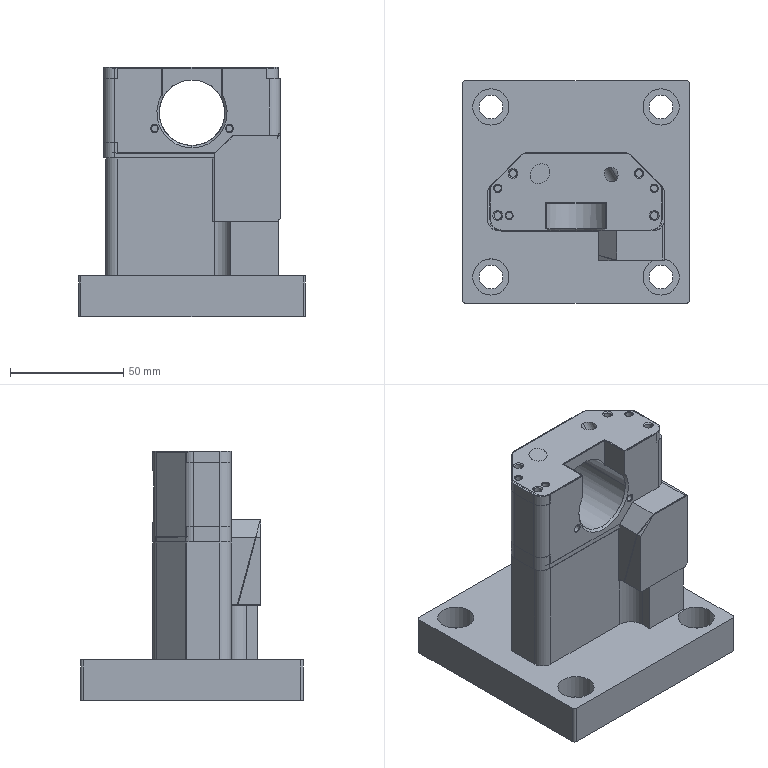NC program | NX | posted with a generic post | part box 100 x 98 x 110 mm
Whole program:
N10 G17 G21 G94 G90
(PLANAR_MILL , TOOL : D80面刀)
N12 T01 M6
N14 G53
N16 G17 G0 G90 X88. Y0. B0. C0. S3500 M3
N18 G43 Z30. H1
N20 Z2.05
N22 G94 G1 Z0.05 F800.
N24 X43.
N26 X-43.
N28 X-88.
N30 Z2.05
N32 G0 Z30.
N34 M5
(ADAPTIVE_MILLING , TOOL : D16-48-D16-100-3T-ROUGH)
N36 T02 M6
N38 G53
N40 G17 G0 G90 X-58.075 Y-25.19 B0. C0. S6500 M3
N42 G43 Z30. H2
N44 Z-24.9
N46 G94 G1 X-57.925 Y-25.183 Z-25.837 F2500.
N48 X-57.775 Y-25.177 Z-26.208
N50 X-57.625 Y-25.171 Z-26.48
N52 X-57.475 Y-25.164 Z-26.7
N54 X-57.325 Y-25.158 Z-26.884
N56 X-57.176 Y-25.152 Z-27.042
N58 X-57.026 Y-25.145 Z-27.18
N60 X-56.876 Y-25.139 Z-27.3
N62 X-56.726 Y-25.133 Z-27.405
N64 X-56.576 Y-25.126 Z-27.498
N66 X-56.426 Y-25.12 Z-27.579
N68 X-56.276 Y-25.114 Z-27.65
N70 X-56.127 Y-25.107 Z-27.71
N72 X-55.977 Y-25.101 Z-27.762
N74 X-55.827 Y-25.095 Z-27.805
N76 X-55.677 Y-25.088 Z-27.839
N78 X-55.527 Y-25.082 Z-27.866
N80 X-55.377 Y-25.075 Z-27.885
N82 X-55.227 Y-25.069 Z-27.896
N84 X-55.077 Y-25.063 Z-27.9
N86 X-52.483 Y-24.953
N88 G3 X-51.072 Y-23.99 R1.616
N90 X-50.404 Y-20.967 R10.918
N92 X-50.046 Y-12.897 R87.213
N94 X-50.001 Y0.166 R855.855
N96 G1 X-50. Y24.239
N98 G2 X-47.644 Y29.928 R8.523
N100 X-42.106 Y33.388 R13.172
N102 X-35.342 Y34.661 R28.151
N104 X-24.774 Y34.98 R145.286
N106 G1 X-12.324 Y34.999
N108 X39.312 Y34.998
N110 G2 X45.036 Y32.543 R8.577
N112 X48.435 Y26.964 R13.333
N114 X49.667 Y20.268 R28.64
N116 X49.98 Y9.775 R147.076
N118 G1 X49.999 Y-2.675
N120 Y-24.311
N122 G2 X47.693 Y-29.819 R8.552
N124 X42.228 Y-33.307 R13.103
N126 X35.398 Y-34.634 R27.707
N128 X24.906 Y-34.969 R139.792
N130 G1 X13.281 Y-34.991
N132 X-39.31 Y-34.998
N134 G2 X-45.115 Y-32.463 R8.58
N136 X-48.122 Y-27.095 R11.826
N138 X-48.966 Y-20.791 R27.513
N140 X-49.036 Y-15.842 R208.259
N142 G1 X-49.029 Y-1.961
N144 X-49.001 Y12.389
N146 G2 X-48.98 Y21.089 R508.483
N148 X-44.643 Y29.357 R11.495
N150 X-38.004 Y32.599 R17.441
N152 X-30.148 Y33.728 R40.171
N154 X-18.527 Y33.985 R219.275
N156 G1 X-8.627 Y33.998
N158 X35.561 Y33.997
N160 G2 X44.259 Y29.758 R11.447
N162 X47.559 Y23.15 R17.233
N164 X48.718 Y15.299 R39.324
N166 X48.986 Y3.079 R220.579
N168 G1 X48.998 Y-6.821
N170 X48.997 Y-20.486
N172 G2 X44.738 Y-29.238 R11.491
N174 X38.283 Y-32.496 R17.176
N176 X30.439 Y-33.693 R38.447
N178 X18.069 Y-33.977 R213.227
N180 G1 X8.169 Y-33.991
N182 X-35.56 Y-33.996
N184 G2 X-41.664 Y-31.998 R10.651
N186 G1 X-42.905 Y-31.48
N188 X-44.056 Y-30.775
N190 X-45.082 Y-29.898
N192 X-45.958 Y-28.872
N194 X-46.663 Y-27.721
N196 X-47.179 Y-26.475
N198 X-47.494 Y-25.162
N200 G2 X-48.002 Y-13.629 R123.608
N202 X-48.015 Y1.606 R886.218
N204 G1 X-48.003 Y10.291
N206 G2 X-47.968 Y18.213 R275.05
N208 X-42.166 Y28.601 R13.302
N210 X-35.036 Y31.664 R20.413
N212 X-26.49 Y32.748 R48.479
N214 X-13.293 Y32.989 R282.507
N216 G1 X-3.393 Y32.998
N218 X32.187 Y32.996
N220 G2 X39.553 Y31.028 R13.666
N222 X45.054 Y24.68 R14.976
N224 X47.217 Y17.129 R26.266
N226 X47.897 Y7.408 R80.681
N228 X47.998 Y-10.216 R882.689
N230 X47.973 Y-18.011 R320.297
N232 X42.252 Y-28.509 R13.323
N234 X35.139 Y-31.617 R20.267
N236 X26.898 Y-32.712 R46.807
N238 X13.252 Y-32.98 R265.456
N240 G1 X3.352 Y-32.991
N242 X-32.11 Y-32.995
N244 G2 X-36.486 Y-32.425 R18.992
N246 G1 X-39.001 Y-32.418
N248 X-40.346 Y-32.312
N250 X-41.728 Y-31.968
N252 X-40.346 Y-32.312
N254 X-39.001 Y-32.418
N256 X-9.236 Y-32.412
N258 X-0.282 Y-32.393
N260 X11.018 Y-32.384
N262 G3 X25.265 Y-32.164 R333.183
N264 X33.82 Y-31.154 R50.803
N266 X40.547 Y-28.463 R20.326
N268 X46.408 Y-20.132 R13.66
N270 X47.244 Y-13.748 R31.907
N272 X47.381 Y-0.7 R293.683
N274 X47.074 Y12.045 R211.801
N276 X45.853 Y20.115 R41.147
N278 X42.614 Y26.753 R18.068
N280 X35.102 Y31.424 R13.688
N282 X28.566 Y32.254 R32.76
N284 X15.968 Y32.396 R326.258
N286 G1 X-4.782 Y32.397
N288 G3 X-23.156 Y32.26 R693.507
N290 X-32.265 Y31.482 R66.785
N292 X-39.38 Y29.184 R23.303
N294 X-46.4 Y20.216 R13.699
N296 X-47.242 Y13.908 R31.444
N298 X-47.414 Y4.68 R270.5
N300 G1 X-47.494 Y4.315
N302 X-47.6 Y2.969
N304 Y-23.818
N306 Y2.969
N308 X-47.494 Y4.315
N310 G3 X-46.534 Y10.33 R29.295
N312 G2 X-45.911 Y16.496 R71.557
N314 X-43.095 Y23.454 R15.66
N316 X-36.299 Y28.647 R16.486
N318 X-28.406 Y30.675 R29.752
N320 X-18.531 Y31.301 R92.666
N322 X-0.456 Y31.397 R915.333
N324 G1 X15.419 Y31.396
N326 G2 X27.492 Y31.242 R280.899
N328 X33.574 Y30.416 R29.057
N330 X42.537 Y23.47 R14.783
N332 X45.241 Y16.027 R23.602
N334 X46.184 Y7.161 R58.748
N336 X46.253 Y-12.185 R283.781
N338 X45.467 Y-18.349 R30.55
N340 X38.488 Y-27.503 R14.785
N342 X30.896 Y-30.25 R23.745
N344 X21.652 Y-31.194 R61.005
N346 X6.054 Y-31.387 R439.644
N348 G1 X-5.768 Y-31.414
N350 X-6.133 Y-31.496
N352 X-7.344 Y-31.998
N354 X-8.656 Y-32.312
N356 X-10.001 Y-32.418
N358 X-8.656 Y-32.312
N360 X-7.344 Y-31.998
N362 G2 X-5.722 Y-31.351 R17.199
N364 X-1.746 Y-30.922 R22.329
N366 X10.769 Y-30.774 R388.142
N368 G3 X23.588 Y-30.46 R224.645
N370 X32.036 Y-29.229 R44.944
N372 X39.059 Y-25.944 R19.641
N374 X44.364 Y-18.103 R15.397
N376 X45.548 Y-10.941 R31.143
N378 X45.724 Y1.28 R168.759
N380 X45.168 Y11.986 R107.119
N382 X43.408 Y19.641 R31.315
N384 X38.702 Y26.418 R16.297
N386 X31.638 Y29.77 R16.943
N388 X24.126 Y30.651 R40.541
N390 X10.852 Y30.795 R369.941
N392 G1 X-0.973 Y30.796
N394 G3 X-19.722 Y30.653 R701.226
N396 X-29.206 Y29.854 R71.207
N398 X-36.617 Y27.525 R25.073
N400 X-44.305 Y18.484 R15.388
N402 X-45.625 Y12.257 R32.254
N404 G2 X-46.277 Y7.6 R70.9
N406 X-46.662 Y6.874 R3.295
N408 G1 X-47.179 Y5.627
N410 X-46.662 Y6.874
N412 G3 X-45.378 Y9.898 R8.871
N414 G2 X-44.132 Y15.049 R332.181
N416 X-40.97 Y21.631 R18.462
N418 X-33.549 Y27.073 R17.846
N420 X-25.483 Y29.063 R32.066
N422 X-14.633 Y29.71 R102.283
N424 X1.642 Y29.795 R879.079
N426 G1 X13.867 Y29.79
N428 G2 X24.738 Y29.551 R179.675
N430 X31.674 Y28.388 R29.743
N432 X41.122 Y20.485 R16.054
N434 X43.716 Y12.678 R26.107
N436 X44.611 Y3.053 R67.824
N438 X44.513 Y-10.066 R135.948
N440 X43.272 Y-16.99 R27.963
N442 X35.554 Y-26.062 R16.036
N444 X27.831 Y-28.672 R25.845
N446 X18.434 Y-29.592 R66.11
N448 X4.343 Y-29.807 R497.152
N450 G3 X-3.02 Y-30.111 R78.907
N452 X-4.413 Y-30.392 R4.781
N454 X-4.946 Y-30.776 R2.898
N456 G1 X-6.097 Y-31.481
N458 X-4.946 Y-30.776
N460 G2 X-3.579 Y-30.029 R2.786
N462 X0.811 Y-29.405 R21.604
N464 X10.981 Y-29.154 R224.346
N466 G3 X22.594 Y-28.693 R153.526
N468 X30.978 Y-27.112 R38.213
N470 X38.201 Y-22.942 R18.651
N472 X42.76 Y-15.102 R17.272
N474 X43.917 Y-7.555 R35.055
N476 X43.582 Y8.776 R109.392
N478 X41.811 Y16.889 R34.002
N480 X36.94 Y24.18 R17.621
N482 X29.545 Y27.926 R18.037
N484 X21.98 Y28.978 R38.71
N486 X9.534 Y29.192 R248.694
N488 G1 X-4.041 Y29.189
N490 G3 X-19.113 Y28.947 R342.861
N492 X-28.339 Y27.861 R56.12
N494 X-35.848 Y24.899 R22.996
N496 X-42.4 Y17.032 R17.254
N498 X-44.286 Y11.46 R46.053
N500 G2 X-45.105 Y9.071 R21.366
N502 X-45.957 Y8.024 R9.54
N504 G1 X-46.192 Y7.641
N506 X-45.957 Y8.024
N508 G3 X-44.671 Y9.587 R17.572
N510 X-43.156 Y12.716 R21.635
N512 G2 X-40.515 Y17.994 R33.226
N514 X-31.669 Y25.25 R19.09
N516 X-23.187 Y27.404 R33.088
N518 X-12.864 Y28.081 R97.693
N520 X8.285 Y28.191 R975.394
N522 X20.582 Y27.992 R257.94
N524 X28.15 Y26.962 R38.459
N526 X36.925 Y21.772 R17.29
N528 X41.129 Y14.049 R20.654
N530 X42.701 Y5.205 R41.397
N532 X42.715 Y-8.579 R82.4
N534 X41.064 Y-15.795 R25.588
N536 X32.929 Y-24.532 R17.053
N538 X24.803 Y-27.122 R27.972
N540 X14.95 Y-28.012 R74.106
N542 G1 X4.577 Y-28.271
N544 G3 X-1.596 Y-28.808 R43.09
N546 X-3.304 Y-29.307 R5.919
N548 X-3.92 Y-29.9 R2.525
N550 G1 X-4.604 Y-30.485
N552 G3 X-3.453 Y-29.366 R6.582
N554 G2 X-1.418 Y-28.505 R5.752
N556 X4.213 Y-27.776 R30.746
N558 X14.692 Y-27.407 R682.777
N560 G3 X24.243 Y-26.509 R72.288
N562 X32.136 Y-23.961 R27.021
N564 X40.652 Y-13.963 R17.405
N566 X42.153 Y-5.951 R31.278
N568 X41.589 Y8.785 R68.368
N570 X39.157 Y16.792 R27.793
N572 X28.865 Y25.715 R17.506
N574 X21.303 Y27.2 R32.145
N576 X11.188 Y27.569 R128.167
N578 X-12.511 Y27.476 R954.591
N580 X-23.203 Y26.715 R90.815
N582 X-31.494 Y24.423 R30.688
N584 X-40.378 Y16.412 R19.671
N586 X-42.844 Y11.78 R74.653
N588 G2 X-43.549 Y10.582 R7.886
N590 G1 X-45.034 Y9.097
N592 G3 X-42.66 Y11.506 R59.936
N594 X-40.224 Y14.921 R56.671
N596 G2 X-34.697 Y20.808 R24.828
N598 X-25.848 Y24.843 R25.208
N600 X-16.285 Y26.22 R52.947
N602 X-2.042 Y26.575 R242.346
N604 X15.582 Y26.469 R567.595
N606 X24.011 Y25.677 R55.344
N608 X31.542 Y22.829 R21.085
N610 X38.229 Y14.981 R18.335
N612 X40.64 Y6.344 R30.637
N614 X40.798 Y-7.716 R54.12
N616 X38.513 Y-15.292 R22.648
N618 X30.344 Y-23.037 R17.995
N620 X22.04 Y-25.549 R29.926
N622 X12.41 Y-26.426 R81.776
N624 G3 X3.514 Y-26.885 R211.963
N626 X-1.292 Y-27.721 R23.526
N628 X-2.595 Y-28.312 R4.099
N630 G1 X-2.9 Y-28.641
N632 G3 X-2.988 Y-30.142 R1.601
N634 G1 X-2.826 Y-30.417 Z-27.89
N636 X-2.637 Y-30.674 Z-27.88
N638 X-1.144 Y-32.711 Z-27.8
N640 X-0.441 Y-33.669 F15000.
N642 G3 X2.135 Y-33.676 R1.6
N644 G1 X2.431 Y-33.281
N646 X2.714 Y-32.876
N648 G3 X0.478 Y-30.724 R1.6
N650 G1 X-1.608 Y-31.935 Z-27.876 F2500.
N652 G2 X-2.331 Y-32.114 Z-27.9 R1.608
N654 X-3.556 Y-29.475 R1.6
N656 G3 X-2.764 Y-28.43 R5.177
N658 G2 X-1.281 Y-27.502 R3.929
N660 X3.421 Y-26.44 R18.892
N662 X12.017 Y-25.848 R135.279
N664 G3 X21.419 Y-24.955 R83.666
N666 X29.575 Y-22.469 R29.243
N668 X38.959 Y-11.63 R18.152
N670 X40.404 Y-3.004 R31.419
N672 X39.329 Y9.361 R45.726
N674 X35.867 Y17.296 R22.923
N676 X26.838 Y23.958 R18.293
N678 X18.919 Y25.561 R33.068
N680 X7.98 Y25.966 R131.451
N682 X-12.118 Y25.802 R537.029
N684 X-22.416 Y24.85 R75.463
N686 X-31.087 Y22.04 R29.777
N688 X-38.491 Y15.859 R23.904
N690 G1 X-39.399 Y14.732
N692 X-42.952 Y11.178
N694 X-35.231 Y18.9
N696 X-34.204 Y19.776
N698 X-33.053 Y20.481
N700 G2 X-16.847 Y24.403 R53.299
N702 X-3.737 Y24.94 R165.07
N704 X13.661 Y24.83 R400.813
N706 X22.154 Y23.933 R52.883
N708 X30.047 Y20.735 R21.483
N710 X36.75 Y12.382 R19.159
N712 X39.034 Y3.019 R31.459
N714 X38.623 Y-7.734 R36.684
N716 X34.703 Y-16.317 R19.496
N718 X26.759 Y-22.011 R19.782
N720 X18.125 Y-24.175 R35.49
N722 X8.654 Y-25.008 R145.848
N724 G3 X1.634 Y-25.863 R51.358
N726 X-1.806 Y-27.11 R10.979
N728 X-2.308 Y-27.659 R2.058
N730 X-2.21 Y-29.216 R1.601
N732 G1 X-1.25 Y-30.474 Z-27.85
N734 X-0.279 Y-31.724 Z-27.8
N736 X0.342 Y-32.528 F15000.
N738 G3 X2.727 Y-32.694 R1.6
N740 G1 X3.094 Y-32.339
N742 X3.448 Y-31.972
N744 G3 X1.407 Y-29.581 R1.6
N746 G1 X1.052 Y-29.784
N748 X0.141 Y-30.309 Z-27.833 F2500.
N750 X-0.776 Y-30.822 Z-27.866
N752 G2 X-1.809 Y-30.957 Z-27.9 R1.6
N754 X-2.847 Y-28.554 R1.6
N756 G3 X-2.209 Y-27.453 R10.053
N758 G2 X-0.83 Y-26.395 R3.733
N760 X3.484 Y-25.098 R15.875
N762 X10.306 Y-24.323 R76.522
N764 G3 X19.32 Y-23.309 R98.087
N766 X27.404 Y-20.822 R30.293
N768 X37.303 Y-9.12 R18.643
N770 X38.426 Y0.897 R30.469
N772 X36.476 Y10.863 R31.304
N774 X29.828 Y19.649 R19.128
N776 X21.744 Y23.132 R22.201
N778 X12.893 Y24.188 R50.78
N780 X-3.904 Y24.331 R326.232
N782 X-16.937 Y23.743 R152.148
N784 X-28.391 Y21.447 R56.089
N786 G2 X-29.15 Y21.418 R6.39
N788 G1 X-30.494 Y21.312
N790 X-31.807 Y20.998
N792 X-30.494 Y21.312
N794 G2 X-27.415 Y21.418 R23.178
N796 G3 X-22.295 Y22.035 R67.403
N798 G2 X-5.552 Y23.273 R135.135
N800 X12.07 Y23.176 R288.423
N802 X20.475 Y22.171 R49.577
N804 X28.561 Y18.67 R21.641
N806 X35.217 Y9.865 R19.689
N808 X36.507 Y-6.725 R29.155
N810 X26.812 Y-19.345 R18.612
N812 X18.448 Y-22.16 R30.129
N814 X10.798 Y-23.216 R87.911
N816 G3 X3.406 Y-24.232 R72.861
N818 X-0.699 Y-25.633 R15.013
N820 X-1.825 Y-26.544 R3.007
N822 X-2.324 Y-27.691 R14.952
N824 G1 X-1.8 Y-26.447
N826 G2 X-0.074 Y-25.06 R4.676
N828 X4.501 Y-23.574 R17.516
N830 X11.796 Y-22.519 R97.587
N832 G3 X20.21 Y-21.039 R62.438
N834 X28.083 Y-17.552 R24.828
N836 X35.566 Y-6.543 R18.692
N838 X34.169 Y10.131 R26.417
N840 X23.189 Y20.41 R19.121
N842 X15.162 Y22.219 R32.856
N844 X4.379 Y22.725 R107.919
N846 X-13.612 Y22.309 R242.716
N848 X-22.214 Y21.418 R144.843
N850 G1 X-27.464
N852 X-18.756
N854 G3 X-13.982 Y21.397 R41.826
N856 G2 X6.758 Y21.662 R370.822
N858 X16.396 Y20.905 R70.705
N860 X24.364 Y18.363 R25.782
N862 X33.36 Y7.981 R19.241
N864 X34.119 Y-6.243 R23.313
N866 X25.585 Y-17.223 R18.282
N868 X17.552 Y-20.32 R28.87
N870 X9.246 Y-21.79 R101.081
N872 G3 X2.746 Y-23.143 R45.543
N874 X-0.799 Y-24.808 R11.951
N876 X-1.689 Y-25.925 R2.149
N878 G2 X-1.879 Y-26.615 R6.496
N880 G3 X-1.611 Y-25.636 R11.706
N882 G2 X-0.419 Y-24.321 R3.533
N884 X3.389 Y-22.546 R12.943
N886 X9.411 Y-21.218 R49.003
N888 G3 X17.281 Y-19.685 R101.439
N890 X25.119 Y-16.501 R27.74
N892 X33.759 Y-3.057 R18.367
N894 X30.762 Y11.119 R21.341
N896 X21.567 Y18.587 R19.132
N898 X13.347 Y20.549 R32.24
N900 X2.491 Y21.091 R100.09
N902 X-13.678 Y20.812 R443.152
N904 G2 X-15.598 Y20.822 R13.426
N906 G3 X-17.41 Y21.312 R14.425
N908 G1 X-18.232 Y21.377
N910 X-17.41 Y21.312
N912 X-16.098 Y20.997
N914 G3 X-13.33 Y20.305 R8.12
N916 X-6.37 Y20.074 R68.213
N918 G2 X6.732 Y19.966 R318.395
N920 X15.819 Y18.981 R55.44
N922 X24.003 Y15.723 R23.426
N924 X32.232 Y2.271 R18.829
N926 X29.566 Y-9.861 R17.928
N928 X22.288 Y-16.269 R19.16
N930 X14.52 Y-19.044 R33.917
N932 X7.059 Y-20.653 R500.229
N934 G3 X1.451 Y-22.459 R27.265
N936 X-1.157 Y-24.289 R8.162
N938 X-1.491 Y-25.034 R1.904
N940 X-1.151 Y-26.28 R1.602
N942 G1 X-0.704 Y-26.831
N944 X1.291 Y-29.288 Z-27.8
N946 X1.579 Y-29.637 F15000.
N948 X1.853 Y-29.997
N950 G2 X2.069 Y-31.201 R1.602
N952 G1 X1.969 Y-31.669
N954 X1.854 Y-32.133
N956 G2 X-0.956 Y-32.539 R1.6
N958 X-1.264 Y-31.582 Z-27.832 R1.733 F2500.
N960 G1 X-1.437 Y-29.445 Z-27.9
N962 X-1.693 Y-26.282
N964 G2 X-1.654 Y-25.779 R1.708
N966 G3 X-1.446 Y-24.72 R8.964
N968 G2 X-0.345 Y-23.301 R3.569
N970 X3.463 Y-21.235 R12.662
N972 X9.367 Y-19.604 R48.077
N974 G3 X16.791 Y-17.717 R87.098
N976 X24.308 Y-14.002 R25.468
N978 X31.08 Y3.094 R17.347
N980 X21.206 Y16.175 R17.989
N982 X12.912 Y18.685 R28.065
N984 X2.897 Y19.427 R75.278
N986 X-8.078 Y19.496 R993.355
N988 G2 X-13.635 Y19.881 R37.268
N990 X-14.173 Y20.065 R2.916
N992 G3 X-15.405 Y20.71 R4.816
N994 G2 X-14.173 Y20.065 R4.816
N996 G3 X-11.98 Y19.224 R6.186
N998 X-6.294 Y18.63 R33.85
N1000 X3.284 Y18.398 R939.984
N1002 G2 X12.54 Y17.577 R67.136
N1004 X20.486 Y14.952 R25.878
N1006 X29.324 Y3.105 R17.16
N1008 X24.141 Y-11.893 R15.958
N1010 X16.843 Y-16.213 R23.604
N1012 X9.815 Y-18.38 R65.522
N1014 G3 X3.417 Y-20.361 R53.378
N1016 X-0.432 Y-22.621 R12.905
N1018 X-1.341 Y-23.795 R3.266
N1020 X-1.497 Y-25.053 R5.488
N1022 G1 X-1.395 Y-23.858
N1024 G2 X-0.274 Y-22.216 R3.781
N1026 X3.448 Y-19.926 R12.926
N1028 X8.867 Y-18.078 R46.912
N1030 G3 X15.743 Y-15.888 R84.514
N1032 X22.757 Y-11.88 R24.138
N1034 X28.443 Y-0.387 R15.671
N1036 X22.098 Y12.638 R15.834
N1038 X14.131 Y16.369 R22.021
N1040 X5.234 Y17.638 R47.216
N1042 X-4.839 Y17.992 R397.473
N1044 G2 X-11.116 Y18.587 R41.077
N1046 X-12.889 Y19.115 R7.151
N1048 X-13.701 Y19.775 R11.224
N1050 G1 X-13.828 Y19.853
N1052 G2 X-12.79 Y18.997 R11.827
N1054 G3 X-10.241 Y17.926 R7.482
N1056 X-4.513 Y17.137 R32.596
N1058 G1 X4.005 Y16.68
N1060 G2 X12.539 Y15.51 R49.781
N1062 X20.066 Y12.223 R21.742
N1064 X26.216 Y3.026 R14.99
N1066 X23.155 Y-8.775 R14.124
N1068 X16.809 Y-13.773 R20.13
N1070 X9.788 Y-16.623 R48.956
N1072 G3 X3.696 Y-18.888 R65.067
N1074 X-0.238 Y-21.374 R14.386
N1076 X-1.302 Y-22.771 R4.222
N1078 X-1.4 Y-23.819 R2.711
N1080 G1 X-1.418 Y-24.043
N1082 X-1.391 Y-22.955
N1084 G2 X-0.383 Y-21.234 R3.795
N1086 X3.203 Y-18.686 R12.805
N1088 X8.134 Y-16.625 R45.586
N1090 G3 X14.66 Y-14.032 R76.912
N1092 X20.992 Y-9.716 R22.073
N1094 X25.176 Y-0.481 R14.009
N1096 X20.73 Y10.111 R13.78
N1098 X13.391 Y14.309 R19.213
N1100 X5.083 Y15.894 R38.886
N1102 X-3.472 Y16.481 R341.06
N1104 G2 X-9.575 Y17.3 R38.009
N1106 X-11.864 Y18.125 R8.577
N1108 X-12.846 Y19.045 R31.576
N1110 G1 X-11.722 Y17.946
N1112 G3 X-8.919 Y16.615 R7.957
N1114 X-3.286 Y15.629 R31.8
N1116 G2 X4.713 Y14.881 R781.96
N1118 X12.48 Y13.257 R36.731
N1120 X19.149 Y9.289 R17.544
N1122 X21.218 Y-5.869 R12.293
N1124 X15.841 Y-11.485 R17.357
N1126 X9.38 Y-14.883 R38.561
N1128 G3 X3.525 Y-17.546 R82.193
N1130 X-0.347 Y-20.329 R14.895
N1132 X-1.318 Y-21.736 R4.478
N1134 G1 X-1.4 Y-22.177
N1136 Y-23.152
N1138 X-1.392 Y-21.877
N1140 G2 X-0.254 Y-19.91 R4.448
N1142 X3.448 Y-17.121 R14.728
N1144 X9.287 Y-14.284 R86.518
N1146 G3 X15.302 Y-10.891 R35.734
N1148 X20.163 Y-5.432 R15.861
N1150 X18.785 Y7.467 R11.772
N1152 X12.471 Y12.102 R16.081
N1154 X5.246 Y14.046 R30.05
N1156 X-2.733 Y14.979 R197.411
N1158 G2 X-8.526 Y16.035 R34.841
N1160 X-10.692 Y16.934 R8.396
N1162 G1 X-11.761 Y17.985
N1164 G3 X-10.271 Y16.525 R34.072
N1166 X-7.015 Y15.048 R10.072
N1168 X-1.019 Y13.904 R43.865
N1170 G2 X6.298 Y12.732 R93.7
N1172 X12.824 Y10.336 R22.842
N1174 X17.804 Y5.263 R12.398
N1176 X18.001 Y-3.963 R10.974
N1178 X13.487 Y-9.857 R15.685
N1180 X8.016 Y-13.474 R34.374
N1182 G3 X2.7 Y-16.533 R83.247
N1184 X-0.698 Y-19.503 R13.897
N1186 X-1.376 Y-20.771 R3.152
N1188 X-1.4 Y-22.035 R13.294
N1190 G1 X-1.398 Y-20.76
N1192 G2 X-0.516 Y-18.946 R4.089
N1194 X2.95 Y-15.877 R14.74
N1196 X8.348 Y-12.59 R139.452
N1198 G3 X13.553 Y-8.659 R27.087
N1200 X16.972 Y-2.996 R12.84
N1202 X14.982 Y6.271 R10.625
N1204 X9.104 Y10.71 R14.957
N1206 X2.345 Y12.67 R30.716
N1208 G2 X-4.29 Y13.857 R390.433
N1210 X-8.765 Y15.24 R20.287
N1212 X-9.391 Y15.615 R3.413
N1214 G1 X-10.452 Y16.676
N1216 X-8.871 Y15.118
N1218 G3 X-5.572 Y13.53 R10.685
N1220 X-0.927 Y12.361 R49.351
N1222 G2 X5.263 Y10.825 R59.075
N1224 X10.707 Y8.01 R17.016
N1226 X14.142 Y-2.069 R9.848
N1228 X10.824 Y-8.221 R14.054
N1230 X5.944 Y-12.468 R30.287
N1232 G3 X1.437 Y-15.881 R69.985
N1234 X-1.199 Y-18.936 R11.519
N1236 X-1.4 Y-19.653 R1.982
N1238 G1 Y-20.853
N1240 X-1.398 Y-19.428
N1242 G2 X-0.422 Y-17.399 R4.84
N1244 X2.914 Y-14.122 R18.886
N1246 G3 X7.514 Y-10.42 R135.11
N1248 X11.47 Y-5.713 R17.952
N1250 X11.087 Y4.544 R9.796
N1252 X5.768 Y9.21 R13.792
N1254 X-0.057 Y11.378 R29.906
N1256 G2 X-5.415 Y12.94 R83.924
N1258 X-7.764 Y14.004 R11.25
N1260 G1 X-9.025 Y15.249
N1262 G3 X-7.276 Y13.524 R239.292
N1264 X-4.017 Y11.814 R12.592
N1266 G2 X1.353 Y9.883 R978.529
N1268 X6.311 Y7.108 R17.738
N1270 X9.646 Y-1.121 R9.422
N1272 X7.199 Y-7.572 R13.679
N1274 X3.245 Y-12.141 R31.901
N1276 G3 X-0.165 Y-15.806 R40.413
N1278 X-1.341 Y-17.759 R7.236
N1280 G1 X-1.4 Y-18.129
N1282 Y-19.554
N1284 X-1.399 Y-17.904
N1286 G2 X-0.51 Y-15.839 R5.42
N1288 X2.288 Y-12.404 R27.07
N1290 G3 X5.918 Y-8.025 R38.386
N1292 X7.989 Y-3.243 R12.548
N1294 X6.067 Y4.403 R10.088
N1296 X1.157 Y8.624 R15.403
N1298 X-3.814 Y11.032 R62.799
N1300 G2 X-5.93 Y12.158 R13.778
N1302 G1 X-7.454 Y13.678
N1304 G3 X-5.097 Y11.362 R49.998
N1306 X-1.763 Y9.209 R30.9
N1308 G2 X2.345 Y6.192 R21.217
N1310 X5.274 Y-1.787 R10.076
N1312 X3.343 Y-8.059 R15.457
N1314 X0.498 Y-12.559 R51.982
N1316 G3 X-1.332 Y-15.778 R17.647
N1318 G1 X-1.4 Y-16.158
N1320 Y-18.033
N1322 X-1.399 Y-15.933
N1324 G2 X-0.454 Y-13.433 R8.087
N1326 X1.92 Y-9.278 R704.416
N1328 G3 X3.867 Y-4.023 R16.844
N1330 X2.1 Y3.771 R10.988
N1332 X-1.938 Y8.078 R19.024
N1334 G2 X-2.956 Y8.978 R6.234
N1336 G3 X-3.918 Y10.142 R13.819
N1338 G1 X-5.403 Y11.627
N1340 G2 X-3.042 Y9.116 R27.636
N1342 G3 X-1.355 Y6.715 R20.421
N1344 G2 X1.084 Y2.514 R15.646
N1346 X1.46 Y-5.027 R13.684
N1348 X-0.21 Y-10.076 R28.81
N1350 G3 X-1.366 Y-13.038 R36.097
N1352 G1 X-1.4 Y-13.285
N1354 Y-16.06
N1356 Y-13.06
N1358 G2 X-0.708 Y-10.221 R14.2
N1360 G3 X0.627 Y-5.122 R33.735
N1362 X-0.721 Y3.562 R14.595
N1364 G2 X-1.438 Y5.052 R32.936
N1366 G1 X-1.492 Y5.27
N1368 G2 X-1.153 Y6.459 R1.602
N1370 G1 X-0.681 Y7.05
N1372 X1.294 Y9.522 Z-27.8
N1374 X1.646 Y9.968 F15000.
N1376 X2.012 Y10.403
N1378 G2 X4.675 Y8.83 R1.6
N1380 G1 X4.584 Y8.502
N1382 X4.48 Y8.177
N1384 G2 X2.07 Y7.49 R1.6
N1386 X1.609 Y7.989 Z-27.822 R1.909 F2500.
N1388 G1 X0.17 Y10.01 Z-27.9
N1390 G3 X-1.014 Y10.782 R1.666
N1392 X-2.578 Y8.359 R1.6
N1394 G1 X-2.337 Y7.965
N1396 X-1.821 Y6.718
N1398 X-1.506 Y5.406
N1400 G3 X-1.104 Y2.932 R16.988
N1402 G2 X-1.106 Y-6.452 R23.277
N1404 G1 X-1.4 Y-8.025
N1406 Y-13.125
N1408 G2 X-1.377 Y-6.024 R303.748
N1410 G3 X-1.4 Y-0.655 R41.079
N1412 G1 Y4.061
N1414 X-1.465 Y4.884
N1416 X-1.4 Y4.061
N1418 Y-6.805
N1420 G3 X-0.014 Y-8.404 R1.616
N1422 G1 X2.556 Y-8.775
N1424 X2.704 Y-8.796 Z-27.896
N1426 X2.853 Y-8.817 Z-27.885
N1428 X3.001 Y-8.839 Z-27.866
N1430 X3.15 Y-8.86 Z-27.839
N1432 X3.298 Y-8.881 Z-27.805
N1434 X3.447 Y-8.903 Z-27.762
N1436 X3.595 Y-8.924 Z-27.71
N1438 X3.744 Y-8.946 Z-27.65
N1440 X3.892 Y-8.967 Z-27.579
N1442 X4.04 Y-8.988 Z-27.498
N1444 X4.189 Y-9.01 Z-27.405
N1446 X4.337 Y-9.031 Z-27.3
N1448 X4.486 Y-9.052 Z-27.18
N1450 X4.634 Y-9.074 Z-27.042
N1452 X4.783 Y-9.095 Z-26.884
N1454 X4.931 Y-9.117 Z-26.7
N1456 X5.08 Y-9.138 Z-26.48
N1458 X5.228 Y-9.159 Z-26.208
N1460 X5.377 Y-9.181 Z-25.837
N1462 X5.525 Y-9.202 Z-24.9
N1464 G0 Z30.
N1466 X-58.075 Y-25.184
N1468 Z-67.
N1470 G1 X-57.925 Y-25.178 Z-67.937
N1472 X-57.775 Y-25.171 Z-68.308
N1474 X-57.625 Y-25.165 Z-68.58
N1476 X-57.476 Y-25.159 Z-68.8
N1478 X-57.326 Y-25.153 Z-68.984
N1480 X-57.176 Y-25.147 Z-69.142
N1482 X-57.026 Y-25.14 Z-69.28
N1484 X-56.876 Y-25.134 Z-69.4
N1486 X-56.726 Y-25.128 Z-69.505
N1488 X-56.576 Y-25.122 Z-69.598
N1490 X-56.426 Y-25.115 Z-69.679
N1492 X-56.277 Y-25.109 Z-69.75
N1494 X-56.127 Y-25.103 Z-69.81
N1496 X-55.977 Y-25.097 Z-69.862
N1498 X-55.827 Y-25.091 Z-69.905
N1500 X-55.677 Y-25.084 Z-69.939
N1502 X-55.527 Y-25.078 Z-69.966
N1504 X-55.377 Y-25.072 Z-69.985
N1506 X-55.227 Y-25.066 Z-69.996
N1508 X-55.078 Y-25.06 Z-70.
N1510 X-52.485 Y-24.952
N1512 G3 X-51.072 Y-23.986 R1.616
N1514 X-50.404 Y-20.965 R10.96
N1516 X-50.05 Y-13.19 R84.7
N1518 X-50.001 Y2.864 R999.478
N1520 G1 X-50. Y24.313
N1522 G2 X-47.645 Y29.927 R8.533
N1524 X-42.106 Y33.388 R13.172
N1526 X-35.343 Y34.661 R28.154
N1528 X-25.45 Y34.976 R137.658
N1530 G1 X-11.8 Y34.999
N1532 X39.312
N1534 G2 X45.036 Y32.543 R8.575
N1536 X48.435 Y26.965 R13.333
N1538 X49.667 Y20.268 R28.641
N1540 X49.981 Y9.4 R151.06
N1542 G1 X49.999 Y-3.35
N1544 Y-24.311
N1546 G2 X47.693 Y-29.819 R8.553
N1548 X42.228 Y-33.307 R13.103
N1550 X35.398 Y-34.634 R27.708
N1552 X24.906 Y-34.969 R139.799
N1554 G1 X13.281 Y-34.991
N1556 X-39.31 Y-34.998
N1558 G2 X-44.98 Y-32.594 R8.549
N1560 X-48.042 Y-27.384 R11.601
N1562 X-48.954 Y-21.091 R26.22
N1564 X-49.036 Y-15.842 R161.824
N1566 G1 X-49.028 Y1.038
N1568 X-49.001 Y14.939
N1570 G2 X-48.971 Y21.238 R176.578
N1572 X-44.643 Y29.356 R11.503
N1574 X-38.004 Y32.599 R17.441
N1576 X-30.148 Y33.728 R40.169
N1578 X-17.927 Y33.985 R231.035
N1580 G1 X-6.077 Y33.999
N1582 X35.561 Y33.997
N1584 G2 X44.26 Y29.758 R11.448
N1586 X47.559 Y23.149 R17.234
N1588 X48.718 Y15.298 R39.34
N1590 X48.983 Y3.152 R221.968
N1592 G1 X48.998 Y-7.948
N1594 G2 X48.979 Y-21.01 R947.133
N1596 X44.622 Y-29.334 R11.529
N1598 X38.066 Y-32.556 R17.418
N1600 X30.214 Y-33.708 R39.675
N1602 X18.069 Y-33.978 R220.639
N1604 G1 X8.169 Y-33.991
N1606 X-35.56 Y-33.996
N1608 G2 X-41.661 Y-31.993 R10.485
N1610 G3 X-42.582 Y-31.636 R19.762
N1612 G1 X-43.804 Y-30.951
N1614 X-44.898 Y-30.077
N1616 X-45.836 Y-29.037
N1618 X-46.592 Y-27.858
N1620 X-47.147 Y-26.572
N1622 X-47.486 Y-25.213
N1624 G2 X-48.002 Y-13.629 R121.846
N1626 X-48.024 Y2.141 R962.721
N1628 G1 X-48.003 Y10.516
N1630 G2 X-47.967 Y18.238 R256.326
N1632 X-42.214 Y28.567 R13.298
N1634 X-35.074 Y31.655 R20.357
N1636 X-26.529 Y32.743 R47.874
N1638 X-12.958 Y32.987 R295.441
N1640 G1 X-1.708 Y32.998
N1642 X32.111 Y32.997
N1644 G2 X39.167 Y31.26 R13.839
N1646 X44.855 Y25.082 R14.691
N1648 X47.136 Y17.647 R25.061
N1650 X47.861 Y8.607 R70.764
N1652 X47.996 Y-10.292 R763.72
N1654 X47.973 Y-18.011 R375.996
N1656 X42.252 Y-28.509 R13.322
N1658 X35.139 Y-31.617 R20.267
N1660 X26.748 Y-32.721 R47.2
N1662 X13.102 Y-32.981 R272.711
N1664 G1 X3.202 Y-32.992
N1666 X-32.11 Y-32.996
N1668 G2 X-36.412 Y-32.434 R17.092
N1670 G1 X-39.009 Y-32.418
N1672 G2 X-41.266 Y-32.114 R9.98
N1674 G1 X-41.83 Y-31.91
N1676 G3 X-40.148 Y-32.341 R7.768
N1678 X-36.561 Y-32.418 R36.252
N1680 G1 X-9.537 Y-32.413
N1682 X2.093 Y-32.392
N1684 G3 X22.217 Y-32.276 R945.159
N1686 X31.486 Y-31.59 R76.222
N1688 X38.733 Y-29.488 R25.219
N1690 X45.002 Y-23.735 R13.969
N1692 X46.892 Y-17.684 R17.479
N1694 X47.35 Y-10.052 R61.809
N1696 G1 X47.385 Y-7.953
N1698 X47.483 Y-7.458
N1700 X47.6 Y-5.682
N1702 Y5.847
N1704 G3 X46.821 Y15.037 R238.679
N1706 X45.13 Y22.326 R30.262
N1708 X40.762 Y28.638 R15.28
N1710 X34.432 Y31.584 R14.531
N1712 X27.503 Y32.296 R38.973
N1714 X21.543 Y32.385 R445.464
N1716 G1 X21.029 Y32.418
N1718 X-21.028
N1720 G3 X-29.004 Y31.919 R201.689
N1722 X-36.703 Y30.359 R32.971
N1724 X-43.029 Y26.446 R16.019
N1726 X-46.492 Y19.852 R14.048
N1728 X-47.274 Y13.234 R34.729
N1730 X-47.397 Y8.057 R563.444
N1732 G1 X-47.483 Y7.623
N1734 X-47.6 Y5.848
N1736 Y-23.818
N1738 G2 X-50.711 Y-24.344 R1.6
N1740 G1 X-51.552 Y-21.293 Z-69.9
N1742 X-51.773 Y-20.501 F15000.
N1744 X-51.981 Y-19.706
N1746 X-52.006 Y-19.412
N1748 X-51.803 Y3.652
N1750 G2 X-51.571 Y4.466 R1.61
N1752 X-50.981 Y5.045 Z-69.926 R1.794 F2500.
N1754 G1 X-49.06 Y6.364 Z-70.
N1756 X-48.06 Y7.051
N1758 G3 X-47.397 Y8.057 R1.602
N1760 X-46.739 Y11.341 R104.279
N1762 G2 X-45.948 Y16.733 R141.212
N1764 X-42.994 Y23.631 R15.84
N1766 X-36.134 Y28.727 R16.711
N1768 X-28.303 Y30.704 R30.703
N1770 G3 X-27.2 Y30.906 R4.837
N1772 G1 X-26.232 Y31.383
N1774 X-24.548 Y31.955
N1776 X-22.803 Y32.302
N1778 X-21.606 Y32.38
N1780 X-22.803 Y32.302
N1782 X-24.548 Y31.955
N1784 X-26.232 Y31.383
N1786 G2 X-29.473 Y30.142 R13.037
N1788 G3 X-35.033 Y28.345 R42.923
N1790 X-41.642 Y23.531 R16.709
N1792 X-44.813 Y17.16 R17.826
N1794 X-45.884 Y12.472 R65.962
N1796 G2 X-46.564 Y11.053 R45.451
N1798 G1 X-47.136 Y9.368
N1800 X-46.564 Y11.053
N1802 G3 X-45.17 Y13.876 R91.412
N1804 G2 X-43.296 Y18.308 R73.104
N1806 X-35.249 Y26.467 R18.158
N1808 X-30.647 Y28.491 R46.688
N1810 G1 X-30.396 Y28.654
N1812 X-29.307 Y29.608
N1814 X-27.828 Y30.597
N1816 X-27.357 Y30.829
N1818 X-27.828 Y30.597
N1820 X-29.307 Y29.608
N1822 G2 X-30.777 Y28.351 R25.676
N1824 X-34.274 Y26.313 R82.911
N1826 G3 X-42.673 Y17.508 R20.831
N1828 G1 X-43.828 Y15.239
N1830 X-44.789 Y14.127
N1832 X-45.747 Y12.693
N1834 X-44.789 Y14.127
N1836 G3 X-42.637 Y16.579 R96.766
N1838 G2 X-39.069 Y20.842 R48.468
N1840 X-34.328 Y24.753 R34.166
N1842 G1 X-30.532 Y28.534
N1844 X-30.645 Y28.435
N1846 X-43.397 Y15.684
N1848 G2 X-46.128 Y16.826 R1.6
N1850 X-45.913 Y17.631 Z-69.973 R1.79
N1852 G1 X-44.932 Y19.737 Z-69.9
N1854 X-43.716 Y22.349 F15000.
N1856 G2 X-43.397 Y22.804 R1.671
N1858 G1 X-33.606 Y32.595
N1860 G2 X-30.458 Y34.915 R13.081
N1862 X-25.714 Y36.646 R18.535
N1864 X-22.926 Y36.957 R15.284
N1866 G1 X-15.019 Y37.103
N1868 X-10.076 Y37.187
N1870 X-5.134 Y37.256
N1872 X-0.191 Y37.309
N1874 X4.752 Y37.347
N1876 X16.508 Y37.419
N1878 G2 X17.84 Y36.722 R1.601
N1880 G1 X18.066 Y36.39
N1882 X19.85 Y33.777 Z-70. F2500.
N1884 X20.137 Y33.352
N1886 X20.437 Y32.935
N1888 G3 X21.543 Y32.385 R1.602
N1890 G1 X22.805 Y32.302
N1892 G3 X29.275 Y31.303 R59.567
N1894 G2 X34.76 Y30.113 R24.81
N1896 X42.622 Y23.362 R15.02
N1898 X45.279 Y15.985 R24.37
N1900 X45.873 Y12.511 R136.514
N1902 G3 X46.565 Y11.051 R13.272
N1904 G1 X47.137 Y9.366
N1906 X47.484 Y7.621
N1908 X47.137 Y9.366
N1910 X46.565 Y11.051
N1912 G2 X45.565 Y13.238 R17.241
N1914 G3 X44.133 Y17.986 R428.469
N1916 X40.822 Y24.337 R20.345
N1918 X33.353 Y29.415 R15.897
N1920 X27.512 Y30.798 R40.821
N1922 G2 X26.234 Y31.383 R8.219
N1924 G1 X24.55 Y31.955
N1926 X26.234 Y31.383
N1928 G3 X31.274 Y29.164 R42.252
N1930 G2 X37.267 Y25.653 R20.175
N1932 X42.09 Y19.035 R19.948
N1934 X43.571 Y15.563 R136.321
N1936 G1 X43.699 Y15.37
N1938 X44.79 Y14.126
N1940 G2 X45.845 Y12.512 R23.601
N1942 G3 X44.79 Y14.126 R23.601
N1944 G2 X43.412 Y15.727 R36.552
N1946 X41.429 Y19.102 R67.096
N1948 G3 X36.045 Y25.411 R21.241
N1950 X30.924 Y28.43 R28.312
N1952 G2 X30.202 Y28.824 R5.203
N1954 G1 X29.309 Y29.607
N1956 X27.83 Y30.596
N1958 X29.309 Y29.607
N1960 G3 X33.624 Y26.015 R60.281
N1962 G2 X36.044 Y23.858 R34.377
N1964 G1 X39.359 Y20.527
N1966 G3 X40.629 Y18.455 R50.045
N1968 G1 X43.617 Y15.463
N1970 X30.791 Y28.289
N1972 G2 X31.933 Y31.021 R1.6
N1974 X32.738 Y30.806 Z-69.973 R1.79
N1976 G1 X34.844 Y29.825 Z-69.9
N1978 X37.456 Y28.608 F15000.
N1980 G2 X37.911 Y28.289 R1.671
N1982 G1 X47.002 Y19.199
N1984 G2 X50.429 Y14.448 R18.342
N1986 G1 X50.776 Y13.755
N1988 X51.114 Y13.057
N1990 G2 X52.217 Y9.201 R14.388
N1992 X52.454 Y5.925 R21.737
N1994 G1 X52.42 Y-2.918
N1996 G2 X51.77 Y-4.199 R1.601
N1998 G1 X51.571 Y-4.346
N2000 X49.025 Y-6.225 Z-70. F2500.
N2002 X48.444 Y-6.648
N2004 X47.874 Y-7.085
N2006 G3 X47.385 Y-7.953 R1.605
N2008 X46.746 Y-11.121 R106.601
N2010 G2 X45.965 Y-16.572 R167.052
N2012 X43.201 Y-23.323 R16.049
N2014 X36.296 Y-28.632 R16.525
N2016 X28.551 Y-30.641 R29.65
N2018 X18.827 Y-31.284 R89.298
N2020 X1.578 Y-31.391 R871.395
N2022 G1 X-5.766 Y-31.415
N2024 G3 X-6.269 Y-31.56 R5.195
N2026 X-7.071 Y-32.906 R1.601
N2028 X-6.537 Y-34.15 Z-69.956 R1.677
N2030 G1 X-5.326 Y-35.44 Z-69.9
N2032 X-4.987 Y-35.797 F15000.
N2034 X-4.661 Y-36.165
N2036 G2 X-6.269 Y-38.681 R1.6
N2038 G1 X-6.597 Y-38.615
N2040 X-6.922 Y-38.537
N2042 G2 X-7.415 Y-38.27 R1.668
N2044 G1 X-9.817 Y-36.366
N2046 X-11.265 Y-35.211 Z-69.959 F2500.
N2048 G2 X-11.805 Y-34.057 Z-70. R1.6
N2050 X-10.3 Y-32.418 R1.6
N2052 G1 X-8.744 Y-32.326
N2054 G3 X-6.336 Y-31.599 R10.
N2056 G2 X-5.132 Y-31.223 R3.021
N2058 X0.116 Y-30.86 R39.961
N2060 X13.692 Y-30.754 R943.97
N2062 G3 X25.456 Y-30.316 R150.551
N2064 X33.618 Y-28.766 R36.471
N2066 X40.486 Y-24.747 R17.632
N2068 X44.585 Y-17.843 R16.467
N2070 X45.88 Y-12.34 R50.321
N2072 G2 X46.564 Y-10.887 R13.468
N2074 G1 X47.136 Y-9.203
N2076 X46.564 Y-10.887
N2078 G3 X45.096 Y-13.916 R56.647
N2080 G2 X43.168 Y-18.481 R57.48
N2082 X34.487 Y-26.69 R17.654
N2084 X26.269 Y-28.949 R30.173
N2086 X16.101 Y-29.67 R88.292
N2088 X3.022 Y-29.824 R894.541
N2090 G3 X-3.526 Y-30.172 R57.716
N2092 X-4.678 Y-30.539 R2.403
N2094 G1 X-5.133 Y-30.908
N2096 X-6.238 Y-31.543
N2098 X-5.133 Y-30.908
N2100 G2 X-4.274 Y-30.276 R4.034
N2102 X-1.176 Y-29.578 R11.233
N2104 X6.067 Y-29.222 R79.286
N2106 G3 X19. Y-28.944 R422.043
N2108 X28.23 Y-27.885 R57.883
N2110 X35.892 Y-24.936 R23.733
N2112 X42.221 Y-18.179 R18.476
N2114 X43.831 Y-15.077 R91.194
N2116 G1 X44.789 Y-13.962
N2118 X45.777 Y-12.483
N2120 X44.789 Y-13.962
N2122 G3 X41.115 Y-18.347 R66.06
N2124 G2 X29.611 Y-26.081 R22.728
N2126 X20.544 Y-27.697 R43.989
N2128 X10.43 Y-28.137 R157.245
N2130 G3 X1.263 Y-28.447 R167.318
N2132 X-3.026 Y-29.166 R19.111
N2134 X-3.644 Y-29.57 R1.976
N2136 G2 X-4.58 Y-30.459 R4.367
N2138 G3 X-3.44 Y-29.351 R6.711
N2140 G2 X-1.375 Y-28.491 R5.942
N2142 X4.279 Y-27.772 R31.311
N2144 X14.461 Y-27.424 R600.325
N2146 G3 X24.391 Y-26.547 R78.898
N2148 X33.019 Y-23.85 R29.711
N2150 X39.857 Y-18.538 R24.237
N2152 G2 X41.007 Y-17.321 R20.015
N2154 G1 X42.278 Y-16.472
N2156 X43.616 Y-15.299
N2158 X42.278 Y-16.472
N2160 G2 X39.947 Y-17.961 R38.437
N2162 X35.756 Y-20.875 R151.708
N2164 X24.258 Y-25.296 R32.014
N2166 X13.972 Y-26.37 R74.722
N2168 G3 X4.526 Y-26.803 R451.518
N2170 X-0.94 Y-27.613 R28.732
N2172 X-2.542 Y-28.263 R5.545
N2174 X-3.134 Y-28.996 R2.375
N2176 G1 X-3.582 Y-29.501
N2178 G3 X-2.739 Y-28.39 R5.867
N2180 G2 X-0.983 Y-27.384 R4.658
N2182 X3.924 Y-26.383 R21.372
N2184 X12.968 Y-25.815 R169.716
N2186 G3 X23.185 Y-24.791 R81.844
N2188 X36.384 Y-19.566 R33.797
N2190 G2 X37.678 Y-18.764 R12.485
N2192 G1 X39.204 Y-18.247
N2194 X40.616 Y-17.55
N2196 X39.204 Y-18.247
N2198 G2 X36.68 Y-19.044 R32.482
N2200 G3 X32.27 Y-20.857 R106.455
N2202 G2 X18.698 Y-24.258 R48.786
N2204 X8.988 Y-25.004 R191.659
N2206 G3 X1.879 Y-25.812 R54.225
N2208 X-1.759 Y-27.071 R11.854
N2210 X-2.352 Y-27.735 R1.835
N2212 X-2.475 Y-28.461 R1.617
N2214 G1 X-2.348 Y-30.416
N2216 X-2.143 Y-33.574 Z-69.9
N2218 X-2.121 Y-33.909 F15000.
N2220 X-2.133 Y-34.244
N2222 G2 X-2.352 Y-34.855 R1.629
N2224 G1 X-2.635 Y-35.325
N2226 X-2.932 Y-35.785
N2228 G2 X-5.596 Y-35.566 R1.6
N2230 X-5.623 Y-34.083 Z-69.949 R1.612 F2500.
N2232 G1 X-4.897 Y-32.632 Z-70.
N2234 X-2.906 Y-28.653
N2236 G3 X-2.197 Y-27.419 R9.38
N2238 G2 X-0.557 Y-26.26 R4.296
N2240 X4.077 Y-25.004 R18.017
N2242 X11.661 Y-24.253 R97.221
N2244 G3 X21.871 Y-23.134 R100.259
N2246 X32.506 Y-20.027 R51.658
N2248 G2 X34.585 Y-19.251 R20.202
N2250 G3 X37.245 Y-18.873 R13.141
N2252 G1 X35.774 Y-19.165
N2254 G3 X32.733 Y-19.47 R21.455
N2256 X27.195 Y-20.866 R152.024
N2258 G2 X14.255 Y-22.983 R81.739
N2260 G3 X5.851 Y-23.825 R200.372
N2262 X0.419 Y-25.108 R24.138
N2264 X-1.578 Y-26.234 R7.009
N2266 X-1.903 Y-26.684 R3.204
N2268 G1 X-2.316 Y-27.65
N2270 X-1.814 Y-26.481
N2272 G2 X-0.314 Y-25.195 R4.053
N2274 X4.112 Y-23.675 R15.816
N2276 X11.641 Y-22.646 R72.855
N2278 G3 X22.347 Y-21.251 R122.958
N2280 X30.251 Y-19.451 R156.552
N2282 G1 X31.102 Y-19.282
N2284 X34.
N2286 G3 X28.998 Y-19.304 R137.431
N2288 X23.031 Y-20.15 R77.57
N2290 G2 X10.669 Y-21.739 R245.222
N2292 G3 X3.414 Y-22.978 R51.728
N2294 X-0.574 Y-24.657 R13.276
N2296 X-1.601 Y-25.693 R2.821
N2298 X-1.845 Y-26.549 R5.605
N2300 G1 X-1.604 Y-25.618
N2302 G2 X-0.205 Y-24.179 R4.008
N2304 X3.908 Y-22.434 R14.112
N2306 X11.104 Y-21.135 R53.719
N2308 G3 X24.68 Y-19.282 R367.786
N2310 G1 X29.405
N2312 G3 X20.02 Y-19.298 R736.73
N2314 X7.01 Y-20.828 R109.446
N2316 X1.307 Y-22.57 R23.879
N2318 X-1.19 Y-24.351 R7.51
N2320 X-1.504 Y-25.106 R1.92
N2322 X-1.168 Y-26.218 R1.603
N2324 G1 X-0.685 Y-26.832
N2326 X1.269 Y-29.321 Z-69.9
N2328 X1.567 Y-29.697 F15000.
N2330 X1.854 Y-30.081
N2332 G2 X2.056 Y-31.273 R1.602
N2334 G1 X1.964 Y-31.694
N2336 X1.857 Y-32.113
N2338 G2 X-0.949 Y-32.515 R1.6
N2340 X-1.259 Y-31.557 Z-69.932 R1.733 F2500.
N2342 G1 X-1.434 Y-29.422 Z-70.
N2344 X-1.692 Y-26.275
N2346 G2 X-1.65 Y-25.76 R1.697
N2348 G3 X-1.454 Y-24.757 R7.253
N2350 G2 X-0.354 Y-23.336 R3.469
N2352 X3.321 Y-21.367 R11.96
N2354 X10.385 Y-19.743 R38.62
N2356 G1 X13.87 Y-19.282
N2358 X20.47
N2360 G3 X9.641 Y-19.297 R785.175
N2362 X1.672 Y-21.291 R21.39
N2364 X-1.14 Y-23.448 R7.939
N2366 X-1.431 Y-24.204 R1.882
N2368 G1 X-1.504 Y-25.101
N2370 X-1.399 Y-23.906
N2372 G2 X-0.252 Y-22.269 R3.721
N2374 X3.645 Y-20.076 R11.772
N2376 X6.576 Y-19.282 R16.057
N2378 G1 X10.026
N2380 X5.187 Y-19.295
N2382 G3 X-0.524 Y-21.836 R9.707
N2384 X-1.356 Y-23.09 R2.799
N2386 X-1.424 Y-24.118 R10.591
N2388 G1 X-1.39 Y-23.086
N2390 G2 X-0.473 Y-21.542 R3.275
N2392 X3.553 Y-19.292 R8.563
N2394 G1 X5.395 Y-19.282
N2396 G3 X2.858 Y-19.304 R35.301
N2398 X-1.173 Y-21.781 R5.984
N2400 X-1.4 Y-22.55 R1.894
N2402 G1 Y-23.3
N2404 X-1.381 Y-22.176
N2406 G2 X-0.087 Y-20.361 R3.689
N2408 X1.915 Y-19.302 R5.141
N2410 X3.07 Y-19.282 R19.85
N2412 G3 X1.518 Y-19.304 R19.626
N2414 X-1.212 Y-21.121 R4.089
N2416 X-1.4 Y-21.814 R2.035
N2418 G1 Y-22.414
N2420 X-1.379 Y-21.44
N2422 G2 X0.022 Y-19.701 R3.122
N2424 X1.132 Y-19.282 R2.344
N2426 G1 X1.732
N2428 G3 X0.419 Y-19.353 R5.067
N2430 X-1.249 Y-20.64 R2.658
N2432 X-1.4 Y-21.7 R2.21
N2434 G2 X-1.343 Y-20.731 R3.932
N2436 X0.491 Y-19.282 R2.261
N2438 G1 X0.866
N2440 G3 X-0.423 Y-19.457 R2.763
N2442 X-1.4 Y-21.244 R1.748
N2444 G2 X-0.306 Y-19.382 R1.765
N2446 X0.123 Y-19.294 R5.18
N2448 X1.823 Y-20.479 R1.616
N2450 G1 X2.574 Y-23.238
N2452 X2.613 Y-23.382 Z-69.996
N2454 X2.653 Y-23.527 Z-69.985
N2456 X2.692 Y-23.672 Z-69.966
N2458 X2.731 Y-23.816 Z-69.939
N2460 X2.771 Y-23.961 Z-69.905
N2462 X2.81 Y-24.106 Z-69.862
N2464 X2.85 Y-24.251 Z-69.81
N2466 X2.889 Y-24.395 Z-69.75
N2468 X2.928 Y-24.54 Z-69.679
N2470 X2.968 Y-24.685 Z-69.598
N2472 X3.007 Y-24.83 Z-69.505
N2474 X3.047 Y-24.974 Z-69.4
N2476 X3.086 Y-25.119 Z-69.28
N2478 X3.125 Y-25.264 Z-69.142
N2480 X3.165 Y-25.409 Z-68.984
N2482 X3.204 Y-25.553 Z-68.8
N2484 X3.243 Y-25.698 Z-68.58
N2486 X3.283 Y-25.843 Z-68.308
N2488 X3.322 Y-25.988 Z-67.937
N2490 X3.362 Y-26.132 Z-67.
N2492 G0 Z30.
N2494 M5
(FLOOR_WALL , TOOL : D12-36-D12-120-3T-FINISH)
N2496 T06 M6
N2498 G53
N2500 G17 G0 G90 X-34.7 Y-32.818 B0. C0. S4500 M3
N2502 G43 Z30. H6
N2504 Z3.
N2506 G94 G1 Z0. F800.
N2508 Y-29.818
N2510 Y15.33
N2512 X-31.511 Y18.518
N2514 X-28.167
N2516 Y-29.818
N2518 X-21.633
N2520 Y18.518
N2522 X-16.395
N2524 X-15.1 Y17.223
N2526 Y-29.818
N2528 Y-32.818
N2530 Z3.
N2532 G0 Z30.
(PLANAR_MILL_1 , TOOL : D12-36-D12-120-3T-FINISH)
N2534 X16.918 Y-22.682
N2536 Z-25.
N2538 G1 Z-28.
N2540 Y-10.682
N2542 X-3.4
N2544 Y4.062
N2546 G3 X-5.333 Y8.729 R6.6
N2548 G1 X-14.09 Y17.485
N2550 G3 X-18.756 Y19.418 R6.6
N2552 G1 X-27.5
N2554 X-24.564 Y22.354
N2556 G2 X-21.029 Y23.818 R5.
N2558 G1 X21.029
N2560 G2 X24.564 Y22.354 R5.
N2562 G1 X37.536 Y9.383
N2564 G2 X39. Y5.847 R5.
N2566 G1 Y-5.682
N2568 G2 X34. Y-10.682 R5.
N2570 G1 X16.918
N2572 Y-3.482
N2574 X3.8
N2576 Y4.062
N2578 G3 X-0.242 Y13.82 R13.8
N2580 G1 X-3.04 Y16.618
N2582 X20.118
N2584 X31.8 Y4.936
N2586 Y-3.482
N2588 X16.918
N2590 Y3.718
N2592 X11.
N2594 Y4.062
N2596 G3 X10.305 Y9.418 R21.
N2598 G1 X17.135
N2600 X22.835 Y3.718
N2602 X16.918
N2604 Y-22.682
N2606 Z-25.
N2608 G0 Z30.
(PLANAR_MILL_1_COPY , TOOL : D12-36-D12-120-3T-FINISH)
N2610 X-51.445 Y-0.143
N2612 Z-26.
N2614 G1 Z-28.
N2616 X-43.667 Y7.635
N2618 X-33.817 Y17.485
N2620 G2 X-29.15 Y19.418 R6.6
N2622 G1 X-18.756
N2624 G2 X-14.09 Y17.485 R6.6
N2626 G1 X-5.333 Y8.729
N2628 G2 X-3.4 Y4.062 R6.6
N2630 G1 Y-23.818
N2632 Y-34.818
N2634 Z-26.
N2636 G0 Z30.
N2638 M5
(DRILLING , TOOL : 倒角D8-90度)
N2640 T03 M6
N2642 G53
N2644 G17 G0 G90 X-24. Y1.318 B0. C0. S2000 M3
N2646 G43 Z30. H3
N2648 G94 G81 G99 Z-3.1 F200. R3.
N2650 G80
N2652 G0 X-24. Y1.318 Z30.
(DRILLING_COPY , TOOL : 倒角D8-90度)
N2654 X26.
N2656 G81 Z-31.1 F200. R-25.
N2658 G80
N2660 G0 X26. Y1.318 Z30.
N2662 M5
(DRILLING_COPY_1 , TOOL : 钻头D5.1-62-92)
N2664 T04 M6
N2666 G53
N2668 G17 G0 G90 X-24. Y1.318 B0. C0. S2000 M3
N2670 G43 Z30. H4
N2672 G94 G83 G99 Z-20. F200. Q3. R3.
N2674 G80
N2676 G0 X-24. Y1.318 Z30.
(DRILLING_COPY_COPY , TOOL : 钻头D5.1-62-92)
N2678 X26.
N2680 G83 Z-48. F200. Q3. R-25.
N2682 G80
N2684 G0 X26. Y1.318 Z30.
N2686 M5
(DRILLING_COPY_1_COPY , TOOL : 上排M6-23-D6-63)
N2688 T05 M6
N2690 G53
N2692 G17 G0 G90 X-24. Y1.318 B0. C0. S400 M3
N2694 G43 Z30. H5
N2696 G84 G94 G99 Z-15. F400. R3.
N2698 G80
N2700 G0 X-24. Y1.318 Z30.
(DRILLING_COPY_COPY_COPY , TOOL : 上排M6-23-D6-63)
N2702 X26.
N2704 G84 Z-43. F400. R-25.
N2706 G80
N2708 G0 X26. Y1.318 Z30.
N2710 M5
N2712 M2